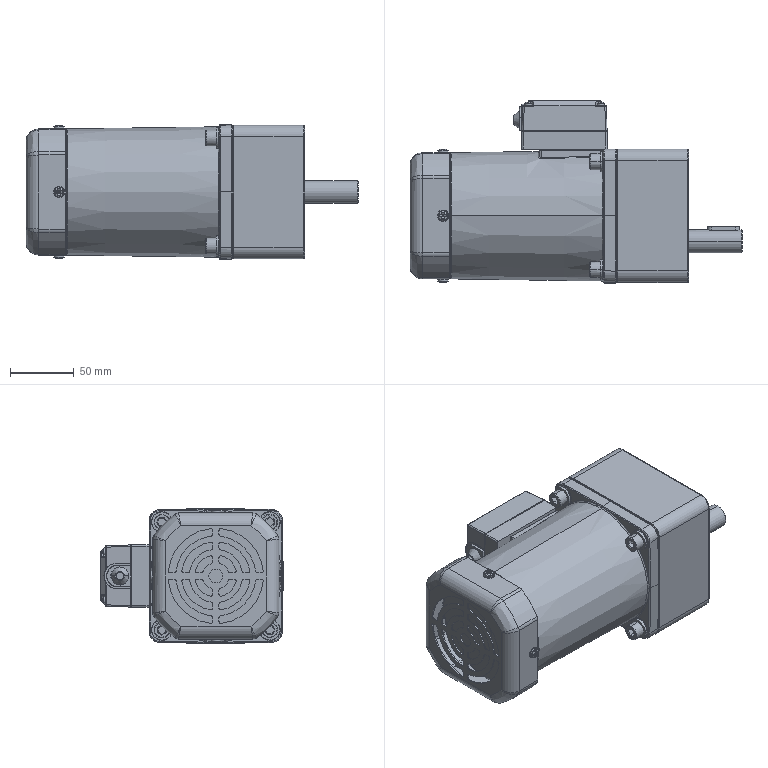Part | SolidWorks | features BaseBody 4 | 4 solids | 1555 faces | box 261 x 143.386 x 105.972 mm | volume 1074405 mm3 | spline 597 | cylinder 462 | plane 429 | cone 59 | torus 8 | commonest cylinder face diameters 0.5 x64 3 x54 4 x44 8 x44 1 x24 2 x17